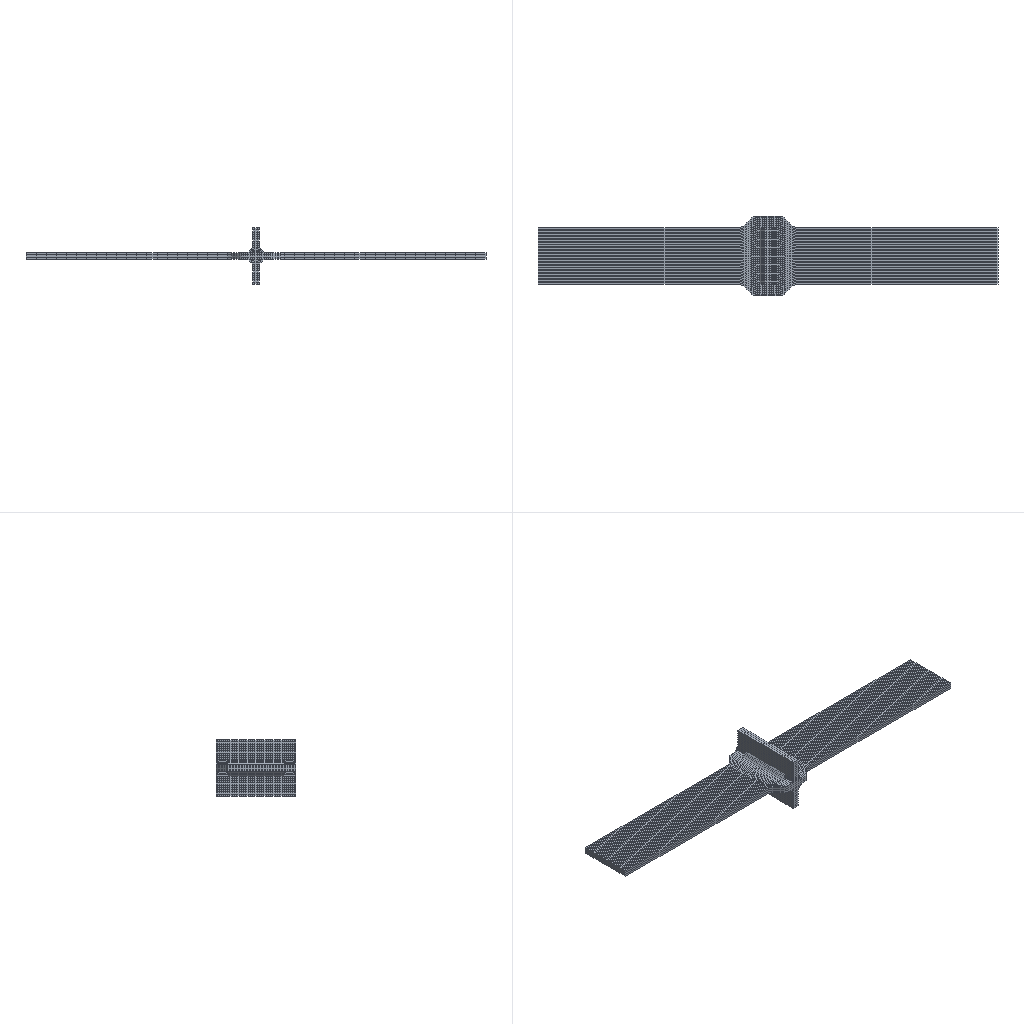Simulation study | abaqus
Set-up summary:
category,name,step,type,value,unit,region
solver,abaqus
solver,version,,,Abaqus/Standard 3DEXPERIENCE R2017x
units,not stated in the deck,,not stated
analysis,deck,,transient,transient
load_step,Step-1,Step-1,transient
load_step,requested,,,1
mesh,nodes,,,16573
mesh,elements,,,12430
element_type,R3D3,,rigid,6
element_type,R3D4,,rigid,1271
element_type,C3D8RT,,solid,11153
load,load commands in deck,,count,3
bc,support commands in deck,,count,7
material,MATERIAL-1,,in results
material,RIG,,in results
check,setup vs results,,match,"per instance, exact: element labels, types and connectivity; labels of the nodes the elements use; coordinates of those nodes at SINGLE_PRECISION in 1 of 3 instance(s)"
Abaqus input file, long lists of numbers shortened:
*Heading
** Job name: [REDACTED] Model name: Model-1-Copy-chongji-Copy
** Generated by: Abaqus/CAE 2017
*Preprint, echo=NO, model=NO, history=NO, contact=NO
**
** PARTS
**
*Part, name=Part-1
*Node
      1,  -10.243,          70.,           6.
      2,  -10.243,          70.,           0.
** (14566 more lines like these left out)
*Element, type=C3D8RT
1,  134, 1857,  129,    1,  135, 1859,  136,    6
2, 1857, 1858,  130,  129, 1859, 1860,  137,  136
** (10676 more lines like these left out)
*Nset, nset=Set-5, generate
     1,  14568,      1
*Elset, elset=Set-5, generate
     1,  10678,      1
** Section: Section-1
*Solid Section, elset=Set-5, material=Material-1
,
*End Part
**
*Part, name=add
*Node
      1,   4.243,          60.,           6.
      2,   4.243,          10.,           6.
** (726 more lines like these left out)
*Element, type=C3D8RT
  1, 273, 276,  96,  95, 441, 444, 299, 300
  2, 276, 275,  97,  96, 444, 443, 298, 299
** (473 more lines like these left out)
*Nset, nset=Set-5, generate
   1,  728,    1
*Elset, elset=Set-5, generate
   1,  475,    1
** Section: Section-1
*Solid Section, elset=Set-5, material=Material-1
,
*End Part
**
*Part, name=rig
*Node
      1,          1.5,           0.,           0.
      2,          1.5,          10.,           0.
** (1274 more lines like these left out)
*Element, type=R3D4
   1,    1,   33,  101,   34
   2,   33,   32,  102,  101
** (1269 more lines like these left out)
*Element, type=R3D3
1024, 1143, 1090, 1098
1025, 1148, 1149, 1101
** (4 more lines like these left out)
*Node
   1277,           0.,          10.,  9.18485073e-17
*Nset, nset=rig-RefPt_, internal
1277,
*Elset, elset=rig, generate
    1,  1277,     1
*End Part
**
**
** ASSEMBLY
**
*Assembly, name=Assembly
**
*Instance, name=Part-1-1, part=Part-1
    -2.121,         -10.,     -8.121
*End Instance
**
*Instance, name=add-1, part=add
    -2.121,         -10.,     -8.121
*End Instance
**
*Instance, name=rig-1, part=rig
2.511,  -1.33226762955019e-15, -1.122
2.511,  -1.33226762955019e-15, -1.122, 3.474, 0.1915, -1.314, 92.181
*End Instance
**
*Nset, nset=Set-1, instance=Part-1-1
    13,    14,    15,    16,    33,    34,    44,    45,    49,    50,    54,    55,    65,    70,    71,    76
    82,    91,   213,   214,   215,   216,   217,   218,   219,   220,   221,   222,   223,   224,   225,   226
** (52 more lines like these left out)
*Elset, elset=Set-1, instance=Part-1-1, generate
 10213,  10637,      1
*Nset, nset=Set-4, instance=Part-1-1
    99,   100,   103,   104,   109,   110,   111,   112,   115,   116,   119,   120,   125,   126,   127,   128
  1024,  1025,  1026,  1027,  1028,  1029,  1030,  1031,  1032,  1033,  1034,  1035,  1036,  1037,  1038,  1039
** (397 more lines like these left out)
*Elset, elset=Set-4, instance=Part-1-1
 4108, 4109, 4110, 4111, 4112, 4113, 4114, 4115, 4116, 4117, 4118, 4119, 4120, 4121, 4122, 4123
 4124, 4125, 4126, 4127, 4128, 4129, 4130, 4131, 4132, 4133, 4134, 4135, 4136, 4137, 4138, 4139
** (276 more lines like these left out)
*Nset, nset=Set-5, instance=Part-1-1, generate
     1,  14568,      1
*Elset, elset=Set-5, instance=Part-1-1, generate
     1,  10678,      1
*Nset, nset=Set-6, instance=add-1, generate
   1,  728,    1
*Elset, elset=Set-6, instance=add-1, generate
   1,  475,    1
*Nset, nset=Set-7, instance=Part-1-1, generate
     1,  14568,      1
*Nset, nset=Set-7, instance=add-1, generate
   1,  728,    1
*Elset, elset=Set-7, instance=Part-1-1, generate
     1,  10678,      1
*Elset, elset=Set-7, instance=add-1, generate
   1,  475,    1
*Nset, nset=Set-8, instance=Part-1-1
    13,    14,    15,    16,    33,    34,    44,    45,    49,    50,    54,    55,    65,    70,    71,    76
    82,    91,   213,   214,   215,   216,   217,   218,   219,   220,   221,   222,   223,   224,   225,   226
** (52 more lines like these left out)
*Nset, nset=Set-8, instance=add-1, generate
   1,  728,    1
*Elset, elset=Set-8, instance=Part-1-1, generate
 10213,  10637,      1
*Elset, elset=Set-8, instance=add-1, generate
   1,  475,    1
*Nset, nset=Set-9, instance=add-1, generate
   1,  728,    1
*Elset, elset=Set-9, instance=add-1, generate
   1,  475,    1
*Nset, nset=Set-10, instance=Part-1-1, generate
     1,  14568,      1
*Nset, nset=Set-10, instance=add-1, generate
   1,  728,    1
*Elset, elset=Set-10, instance=Part-1-1, generate
     1,  10678,      1
*Elset, elset=Set-10, instance=add-1, generate
   1,  475,    1
*Nset, nset=Set-11, instance=Part-1-1
  109,  110,  111,  112,  125,  126,  127,  128, 1248, 1249, 1250, 1251, 1252, 1253, 1254, 1255
 1256, 1257, 1258, 1259, 1260, 1261, 1262, 1263, 1264, 1265, 1266, 1267, 1268, 1269, 1270, 1271
** (17 more lines like these left out)
*Elset, elset=Set-11, instance=Part-1-1
 4811, 4812, 4813, 4814, 4815, 4816, 4817, 4818, 4819, 4820, 4821, 4822, 4823, 4824, 4825, 4826
 4827, 4828, 4829, 4830, 4831, 4832, 4833, 4834, 4835, 4836, 4837, 4838, 4839, 4840, 4841, 4842
** (12 more lines like these left out)
*Nset, nset=Set-12, instance=Part-1-1, generate
     1,  14568,      1
*Nset, nset=Set-12, instance=add-1, generate
   1,  728,    1
*Elset, elset=Set-12, instance=Part-1-1, generate
     1,  10678,      1
*Elset, elset=Set-12, instance=add-1, generate
   1,  475,    1
*Nset, nset=Set-13, instance=rig-1
 1277,
*Nset, nset=Set-14, instance=rig-1
 1277,
*Nset, nset=Set-15, instance=rig-1
 1277,
*Elset, elset=_Surf-1_S4, internal, instance=Part-1-1
     3,     6,     9,    12,    15,    18,    21,    24,    27,    30,    33,    36,    39,    42,    45,    48
    51,    54,    57,    60,    63,    66,    69,    72,    75,    78,    81,    84,    87,    90,    93,    96
** (63 more lines like these left out)
*Elset, elset=_Surf-1_S6, internal, instance=Part-1-1
     1,     4,     7,    10,    13,    16,    19,    22,    25,    28,    31,    34,    37,    40,    43,    46
    49,    52,    55,    58,    61,    64,    67,    70,    73,    76,    79,    82,    85,    88,    91,    94
** (50 more lines like these left out)
*Elset, elset=_Surf-1_S3, internal, instance=Part-1-1
  445,  446,  447,  556,  557,  558,  667,  668,  669,  781,  784,  787,  790,  793,  871,  874
  877,  880,  883,  892,  895,  898,  901,  904,  982,  985,  988,  991,  994, 1003, 1006, 1009
** (38 more lines like these left out)
*Elset, elset=_Surf-1_S5, internal, instance=Part-1-1
   553,   554,   555,   664,   665,   666,   775,   776,   777,   783,   786,   789,   792,   795,   873,   876
   879,   882,   885,   894,   897,   900,   903,   906,   984,   987,   990,   993,   996,  1005,  1008,  1011
** (31 more lines like these left out)
*Elset, elset=_Surf-1_S1, internal, instance=Part-1-1
     1,     2,     3,     4,     5,     6,   223,   224,   225,   226,   227,   228,  3553,  3554,  3555,  3556
  3557,  3558,  3559,  3560,  3561,  3562,  3563,  3564,  3565,  3566,  3567,  3568,  3569,  3570,  3571,  3572
** (133 more lines like these left out)
*Elset, elset=_Surf-1_S2, internal, instance=Part-1-1
   217,   218,   219,   220,   221,   222,   439,   440,   441,   442,   443,   444,  1999,  2000,  2001,  2002
  2003,  2004,  2005,  2006,  2007,  2008,  2009,  2010,  2011,  2012,  2013,  2014,  2015,  2016,  2017,  2018
** (147 more lines like these left out)
*Surface, type=ELEMENT, name=Surf-1
_Surf-1_S4, S4
_Surf-1_S6, S6
_Surf-1_S2, S2
_Surf-1_S3, S3
_Surf-1_S5, S5
_Surf-1_S1, S1
*Elset, elset=_Surf-2_S4, internal, instance=Part-1-1
     3,     6,     9,    12,    15,    18,    21,    24,    27,    30,    33,    36,    39,    42,    45,    48
    51,    54,    57,    60,    63,    66,    69,    72,    75,    78,    81,    84,    87,    90,    93,    96
** (63 more lines like these left out)
*Elset, elset=_Surf-2_S6, internal, instance=Part-1-1
     1,     4,     7,    10,    13,    16,    19,    22,    25,    28,    31,    34,    37,    40,    43,    46
    49,    52,    55,    58,    61,    64,    67,    70,    73,    76,    79,    82,    85,    88,    91,    94
** (50 more lines like these left out)
*Elset, elset=_Surf-2_S3, internal, instance=Part-1-1
  445,  446,  447,  556,  557,  558,  667,  668,  669,  781,  784,  787,  790,  793,  871,  874
  877,  880,  883,  892,  895,  898,  901,  904,  982,  985,  988,  991,  994, 1003, 1006, 1009
** (38 more lines like these left out)
*Elset, elset=_Surf-2_S5, internal, instance=Part-1-1
   553,   554,   555,   664,   665,   666,   775,   776,   777,   783,   786,   789,   792,   795,   873,   876
   879,   882,   885,   894,   897,   900,   903,   906,   984,   987,   990,   993,   996,  1005,  1008,  1011
** (31 more lines like these left out)
*Elset, elset=_Surf-2_S1, internal, instance=Part-1-1
     1,     2,     3,     4,     5,     6,   223,   224,   225,   226,   227,   228,  3553,  3554,  3555,  3556
  3557,  3558,  3559,  3560,  3561,  3562,  3563,  3564,  3565,  3566,  3567,  3568,  3569,  3570,  3571,  3572
** (133 more lines like these left out)
*Elset, elset=_Surf-2_S2, internal, instance=Part-1-1
   217,   218,   219,   220,   221,   222,   439,   440,   441,   442,   443,   444,  1999,  2000,  2001,  2002
  2003,  2004,  2005,  2006,  2007,  2008,  2009,  2010,  2011,  2012,  2013,  2014,  2015,  2016,  2017,  2018
** (147 more lines like these left out)
*Surface, type=ELEMENT, name=Surf-2
_Surf-2_S4, S4
_Surf-2_S6, S6
_Surf-2_S2, S2
_Surf-2_S3, S3
_Surf-2_S5, S5
_Surf-2_S1, S1
*Elset, elset=_Surf-5_S4, internal, instance=Part-1-1
     3,     6,     9,    12,    15,    18,    21,    24,    27,    30,    33,    36,    39,    42,    45,    48
    51,    54,    57,    60,    63,    66,    69,    72,    75,    78,    81,    84,    87,    90,    93,    96
** (63 more lines like these left out)
*Elset, elset=_Surf-5_S4, internal, instance=add-1
   4,   7,  10,  13,  16,  17,  18,  19,  23,  26,  29,  32,  35,  36,  37,  38
  42,  45,  48,  51,  54,  55,  56,  57,  61,  64,  67,  70,  73,  74,  75,  76
** (11 more lines like these left out)
*Elset, elset=_Surf-5_S6, internal, instance=Part-1-1
     1,     4,     7,    10,    13,    16,    19,    22,    25,    28,    31,    34,    37,    40,    43,    46
    49,    52,    55,    58,    61,    64,    67,    70,    73,    76,    79,    82,    85,    88,    91,    94
** (50 more lines like these left out)
*Elset, elset=_Surf-5_S3, internal, instance=Part-1-1
  445,  446,  447,  556,  557,  558,  667,  668,  669,  781,  784,  787,  790,  793,  871,  874
  877,  880,  883,  892,  895,  898,  901,  904,  982,  985,  988,  991,  994, 1003, 1006, 1009
** (38 more lines like these left out)
*Elset, elset=_Surf-5_S5, internal, instance=Part-1-1
   553,   554,   555,   664,   665,   666,   775,   776,   777,   783,   786,   789,   792,   795,   873,   876
   879,   882,   885,   894,   897,   900,   903,   906,   984,   987,   990,   993,   996,  1005,  1008,  1011
** (31 more lines like these left out)
*Elset, elset=_Surf-5_S5, internal, instance=add-1
   1,   2,   3,   4,   5,   6,   7,  17,  20,  21,  22,  23,  24,  25,  26,  36
  39,  40,  41,  42,  43,  44,  45,  55,  58,  59,  60,  61,  62,  63,  64,  74
** (11 more lines like these left out)
*Elset, elset=_Surf-5_S1, internal, instance=Part-1-1
     1,     2,     3,     4,     5,     6,   223,   224,   225,   226,   227,   228,  3553,  3554,  3555,  3556
  3557,  3558,  3559,  3560,  3561,  3562,  3563,  3564,  3565,  3566,  3567,  3568,  3569,  3570,  3571,  3572
** (133 more lines like these left out)
*Elset, elset=_Surf-5_S1, internal, instance=add-1, generate
  1,  19,   1
*Elset, elset=_Surf-5_S2, internal, instance=Part-1-1
   217,   218,   219,   220,   221,   222,   439,   440,   441,   442,   443,   444,  1999,  2000,  2001,  2002
  2003,  2004,  2005,  2006,  2007,  2008,  2009,  2010,  2011,  2012,  2013,  2014,  2015,  2016,  2017,  2018
** (147 more lines like these left out)
*Elset, elset=_Surf-5_S2, internal, instance=add-1, generate
 457,  475,    1
*Surface, type=ELEMENT, name=Surf-5
_Surf-5_S4, S4
_Surf-5_S6, S6
_Surf-5_S2, S2
_Surf-5_S3, S3
_Surf-5_S5, S5
_Surf-5_S1, S1
*Elset, elset=_Surf-6_S4, internal, instance=Part-1-1
     3,     6,     9,    12,    15,    18,    21,    24,    27,    30,    33,    36,    39,    42,    45,    48
    51,    54,    57,    60,    63,    66,    69,    72,    75,    78,    81,    84,    87,    90,    93,    96
** (63 more lines like these left out)
*Elset, elset=_Surf-6_S4, internal, instance=add-1
   4,   7,  10,  13,  16,  17,  18,  19,  23,  26,  29,  32,  35,  36,  37,  38
  42,  45,  48,  51,  54,  55,  56,  57,  61,  64,  67,  70,  73,  74,  75,  76
** (11 more lines like these left out)
*Elset, elset=_Surf-6_S6, internal, instance=Part-1-1
     1,     4,     7,    10,    13,    16,    19,    22,    25,    28,    31,    34,    37,    40,    43,    46
    49,    52,    55,    58,    61,    64,    67,    70,    73,    76,    79,    82,    85,    88,    91,    94
** (50 more lines like these left out)
*Elset, elset=_Surf-6_S3, internal, instance=Part-1-1
  445,  446,  447,  556,  557,  558,  667,  668,  669,  781,  784,  787,  790,  793,  871,  874
  877,  880,  883,  892,  895,  898,  901,  904,  982,  985,  988,  991,  994, 1003, 1006, 1009
** (38 more lines like these left out)
*Elset, elset=_Surf-6_S5, internal, instance=Part-1-1
   553,   554,   555,   664,   665,   666,   775,   776,   777,   783,   786,   789,   792,   795,   873,   876
   879,   882,   885,   894,   897,   900,   903,   906,   984,   987,   990,   993,   996,  1005,  1008,  1011
** (31 more lines like these left out)
*Elset, elset=_Surf-6_S5, internal, instance=add-1
   1,   2,   3,   4,   5,   6,   7,  17,  20,  21,  22,  23,  24,  25,  26,  36
  39,  40,  41,  42,  43,  44,  45,  55,  58,  59,  60,  61,  62,  63,  64,  74
** (11 more lines like these left out)
*Elset, elset=_Surf-6_S1, internal, instance=Part-1-1
     1,     2,     3,     4,     5,     6,   223,   224,   225,   226,   227,   228,  3553,  3554,  3555,  3556
  3557,  3558,  3559,  3560,  3561,  3562,  3563,  3564,  3565,  3566,  3567,  3568,  3569,  3570,  3571,  3572
** (133 more lines like these left out)
*Elset, elset=_Surf-6_S1, internal, instance=add-1, generate
  1,  19,   1
*Elset, elset=_Surf-6_S2, internal, instance=Part-1-1
   217,   218,   219,   220,   221,   222,   439,   440,   441,   442,   443,   444,  1999,  2000,  2001,  2002
  2003,  2004,  2005,  2006,  2007,  2008,  2009,  2010,  2011,  2012,  2013,  2014,  2015,  2016,  2017,  2018
** (147 more lines like these left out)
*Elset, elset=_Surf-6_S2, internal, instance=add-1, generate
 457,  475,    1
*Surface, type=ELEMENT, name=Surf-6
_Surf-6_S4, S4
_Surf-6_S6, S6
_Surf-6_S2, S2
_Surf-6_S3, S3
_Surf-6_S5, S5
_Surf-6_S1, S1
*Elset, elset=_m_Surf-3_S4, internal, instance=add-1
   4,   7,  10,  13,  16,  23,  26,  29,  32,  35,  42,  45,  48,  51,  54,  61
  64,  67,  70,  73,  80,  83,  86,  89,  92,  99, 102, 105, 108, 111, 118, 121
** (6 more lines like these left out)
*Elset, elset=_m_Surf-3_S5, internal, instance=add-1
   5,   6,   7,  17,  24,  25,  26,  36,  43,  44,  45,  55,  62,  63,  64,  74
  81,  82,  83,  93, 100, 101, 102, 112, 119, 120, 121, 131, 138, 139, 140, 150
** (5 more lines like these left out)
*Surface, type=ELEMENT, name=m_Surf-3
_m_Surf-3_S4, S4
_m_Surf-3_S5, S5
*Elset, elset=_s_Surf-3_S4, internal, instance=Part-1-1
 2115, 2118, 2121, 2124, 2127, 2130, 2133, 2136, 2139, 2142, 2145, 2148, 2151, 2154, 2157, 2160
 2163, 2166, 2169, 2172, 2175, 2178, 2181, 2184, 2187, 2190, 2193, 2196, 2199, 2202, 2205, 2208
** (7 more lines like these left out)
*Elset, elset=_s_Surf-3_S6, internal, instance=Part-1-1, generate
 3886,  4099,     3
*Surface, type=ELEMENT, name=s_Surf-3
_s_Surf-3_S4, S4
_s_Surf-3_S6, S6
*Rigid Body, ref node=rig-1.rig-RefPt_, elset=rig-1.rig
** Constraint: Constraint-1
*Tie, name=Constraint-1, adjust=yes
m_Surf-3, s_Surf-3
*Elset, elset=__Int-1_gcs0_117_S6, internal, instance=Part-1-1, generate
 6994,  7179,    37
*Surface, type=ELEMENT, name=_Int-1_gcs0_117, internal
__Int-1_gcs0_117_S6, S6
*Elset, elset=__Int-1_gcs0_119_S4, internal, instance=Part-1-1, generate
 6919,  6993,    37
*Surface, type=ELEMENT, name=_Int-1_gcs0_119, internal
__Int-1_gcs0_119_S4, S4
*Elset, elset=__Int-1_gcs0_123_S6, internal, instance=Part-1-1, generate
 6883,  6957,    37
*Surface, type=ELEMENT, name=_Int-1_gcs0_123, internal
__Int-1_gcs0_123_S6, S6
*Elset, elset=__Int-1_gcs0_125_S4, internal, instance=Part-1-1, generate
 7030,  7215,    37
*Surface, type=ELEMENT, name=_Int-1_gcs0_125, internal
__Int-1_gcs0_125_S4, S4
*Elset, elset=__Int-1_gcs0_151_S6, internal, instance=Part-1-1, generate
 3664,  3849,    37
*Surface, type=ELEMENT, name=_Int-1_gcs0_151, internal
__Int-1_gcs0_151_S6, S6
*Elset, elset=__Int-1_gcs0_153_S4, internal, instance=Part-1-1, generate
 3589,  3663,    37
*Surface, type=ELEMENT, name=_Int-1_gcs0_153, internal
__Int-1_gcs0_153_S4, S4
*Elset, elset=__Int-1_gcs0_157_S6, internal, instance=Part-1-1, generate
 3553,  3627,    37
*Surface, type=ELEMENT, name=_Int-1_gcs0_157, internal
__Int-1_gcs0_157_S6, S6
*Elset, elset=__Int-1_gcs0_159_S4, internal, instance=Part-1-1, generate
 3700,  3885,    37
*Surface, type=ELEMENT, name=_Int-1_gcs0_159, internal
__Int-1_gcs0_159_S4, S4
*Elset, elset=__Int-1_gcs0_169_SPOS, internal, instance=rig-1, generate
    1,  1023,     1
*Surface, type=ELEMENT, name=_Int-1_gcs0_169, internal
__Int-1_gcs0_169_SPOS, SPOS
*Elset, elset=__Int-1_gcs0_170_SPOS, internal, instance=rig-1, generate
 1134,  1277,     1
*Surface, type=ELEMENT, name=_Int-1_gcs0_170, internal
__Int-1_gcs0_170_SPOS, SPOS
*Elset, elset=__Int-1_gcs0_172_SNEG, internal, instance=rig-1, generate
    1,  1023,     1
*Surface, type=ELEMENT, name=_Int-1_gcs0_172, internal
__Int-1_gcs0_172_SNEG, SNEG
*Elset, elset=__Int-1_gcs0_173_SNEG, internal, instance=rig-1, generate
 1134,  1277,     1
*Surface, type=ELEMENT, name=_Int-1_gcs0_173, internal
__Int-1_gcs0_173_SNEG, SNEG
*End Assembly
*Amplitude, name=Amp-x, definition=PERIODIC
1,           25.12,              0.,              0.
            50.,              0.
*Amplitude, name=Amp-z, definition=PERIODIC
1,           25.12,              0.,              0.
           116.,              0.
**
** MATERIALS
**
*Material, name=Material-1
*Conductivity
45.,
*Density
 7.8e-09,
*Elastic
210000., 0.3
*Expansion
 1.2e-05,
*Plastic
350.,0.
*Specific Heat
 4.6e+08,
*Material, name=rig
*Density
 7.8e-09,
*Elastic
206000., 0.3
**
** INTERACTION PROPERTIES
**
*Surface Interaction, name=IntProp-1
1.,
*Friction, slip tolerance=0.005
 0.2,
*Surface Behavior, pressure-overclosure=HARD
**
** PHYSICAL CONSTANTS
**
*Physical Constants, absolute zero=-273., stefan boltzmann=5.67e-08
**
** PREDEFINED FIELDS
**
** Name: Predefined Field-1   Type: Stress
*Initial Conditions, type=STRESS, file=D:/_______/_____/_____.___________________
**
** INTERACTIONS
**
** Interaction: Int-1
*Contact
*Contact Inclusions, ALL EXTERIOR
*Contact Property Assignment
 ,  , IntProp-1
*Surface Property Assignment, property=GEOMETRIC CORRECTION
_Int-1_gcs0_117, Circumferential, -16.05, 55., -2.121,  -16.05, 55., -3.121
_Int-1_gcs0_119, Circumferential, -30.192, 55., -2.121,  -30.192, 55., -3.121
_Int-1_gcs0_123, Circumferential, -30.192, -5., -2.121,  -30.192, -5., -3.121
_Int-1_gcs0_125, Circumferential, -16.05, -5., -2.121,  -16.05, -5., -3.121
_Int-1_gcs0_151, Circumferential, 5.808, 55., -8.121,  5.808, 55., -7.121
_Int-1_gcs0_153, Circumferential, 19.95, 55., -8.121,  19.95, 55., -7.121
_Int-1_gcs0_157, Circumferential, 19.95, -5., -8.121,  19.95, -5., -7.121
_Int-1_gcs0_159, Circumferential, 5.808, -5., -8.121,  5.808, -5., -7.121
_Int-1_gcs0_169, Circumferential, 4.424, -2.25075e-15, 3.497,  4.042, -2.06706e-15, 2.573
_Int-1_gcs0_170, Circumferential, 2.221, -1.19325e-15, -1.821,  1.839, -1.00955e-15, -2.745
_Int-1_gcs0_172, Circumferential, 4.424, -2.25075e-15, 3.497,  4.042, -2.06706e-15, 2.573
_Int-1_gcs0_173, Circumferential, 2.221, -1.19325e-15, -1.821,  1.839, -1.00955e-15, -2.745
** ----------------------------------------------------------------
**
** STEP: Step-1
**
*Step, name=Step-1, nlgeom=YES, inc=10000
*Dynamic
0.01,10.,1e-05
**
** BOUNDARY CONDITIONS
**
** Name: BC-1 Type: 对称/反对称/完全固定
*Boundary
Set-11, ENCASTRE
** Name: [REDACTED] : Speed/Angular velocity
*Boundary, type=VELOCITY
Set-13, 2, 2, 5.6
Set-13, 4, 4
Set-13, 5, 5
Set-13, 6, 6
** Name: [REDACTED]
*Boundary, amplitude=Amp-x, type=VELOCITY
Set-14, 1, 1, -1.
** Name: [REDACTED]
*Boundary, amplitude=Amp-z, type=VELOCITY
Set-15, 3, 3, -1.
**
** OUTPUT REQUESTS
**
*Restart, write, frequency=0
**
** FIELD OUTPUT: F-Output-1
**
*Output, field, frequency=1
*Node Output
A, CF, RF, RM, RT, U, V
*Element Output, directions=YES
E, LE, MISES, MISESMAX, MISESONLY, PE, PEEQ, PEMAG, PRESSONLY, S, SSAVG
*Contact Output
CDISP, CSTRESS
**
** HISTORY OUTPUT: H-Output-1
**
*Output, history, variable=PRESELECT
*End Step
Results summary:
result,step,,partial,increments=22 time=0.01139/10.0
result,analysis,,,transient
result,last_loadstep,,,1
result,primary field,,,U
result,reaction total,,FX,0.2076,model units
result,reaction total,,FY,-3.521,model units
result,reaction total,,FZ,-2.992,model units